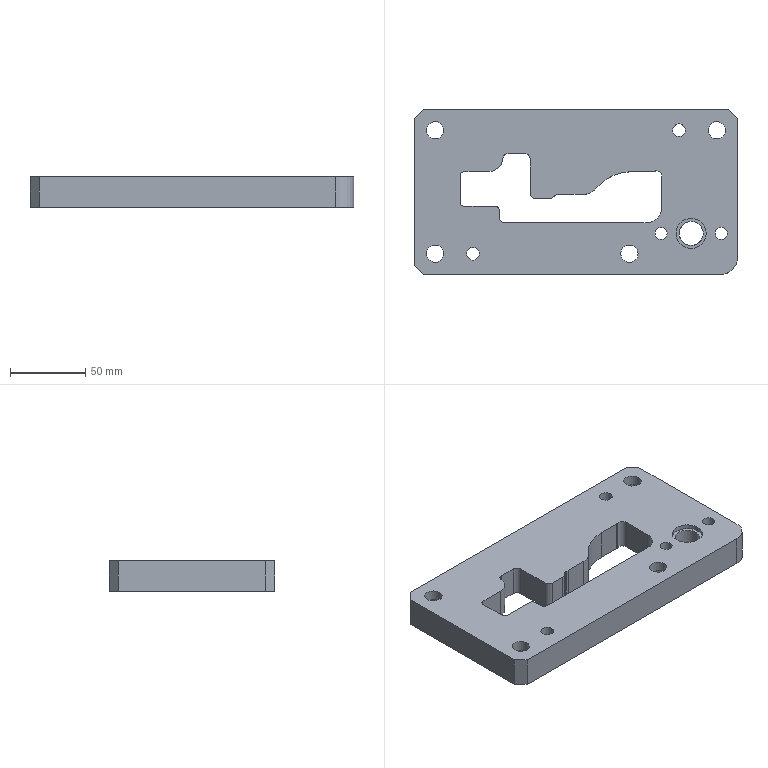Part | STEP file | lll_id222_x_t | 1 solid | 62 faces | box 215 x 110 x 20 mm | volume 372508 mm3 | cylinder 35 | plane 27 | commonest cylinder face diameters 7 x6 5 x4 11.509 x4 18.007 x4 8 x2 8.505 x2